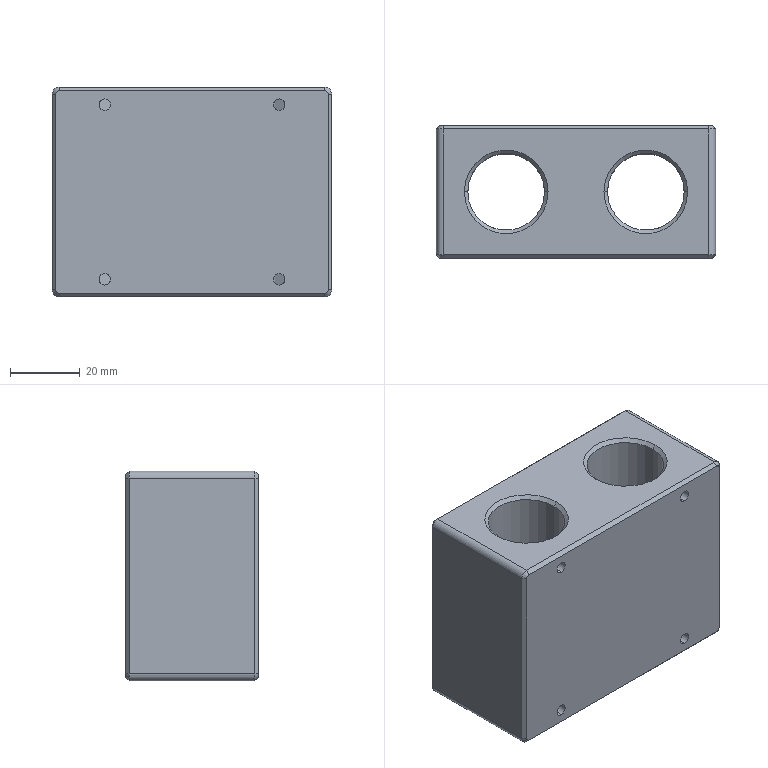Part | STEP file | Guide wheel mechanism revised.sldasm-Part-40 | 1 solid | 58 faces | box 80 x 38 x 60 mm | volume 135299 mm3 | cone 22 | cylinder 22 | plane 14 | commonest cylinder face diameters 3.3 x8 5 x6 4 x4 22 x4